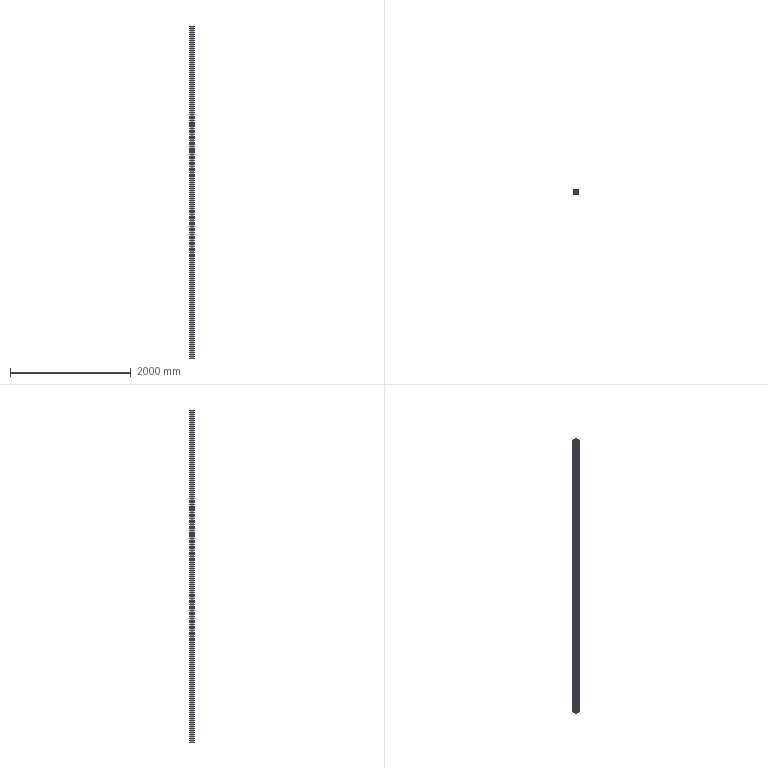Part | SolidWorks | features Extrusion 1 | 1 solid | 307 faces | box 80 x 80 x 5500 mm | volume 9576060 mm3 | plane 194 | cylinder 113 | commonest cylinder face diameters 2 x52 0.4 x16 0.6 x16 4 x9 5 x8 6.8 x8